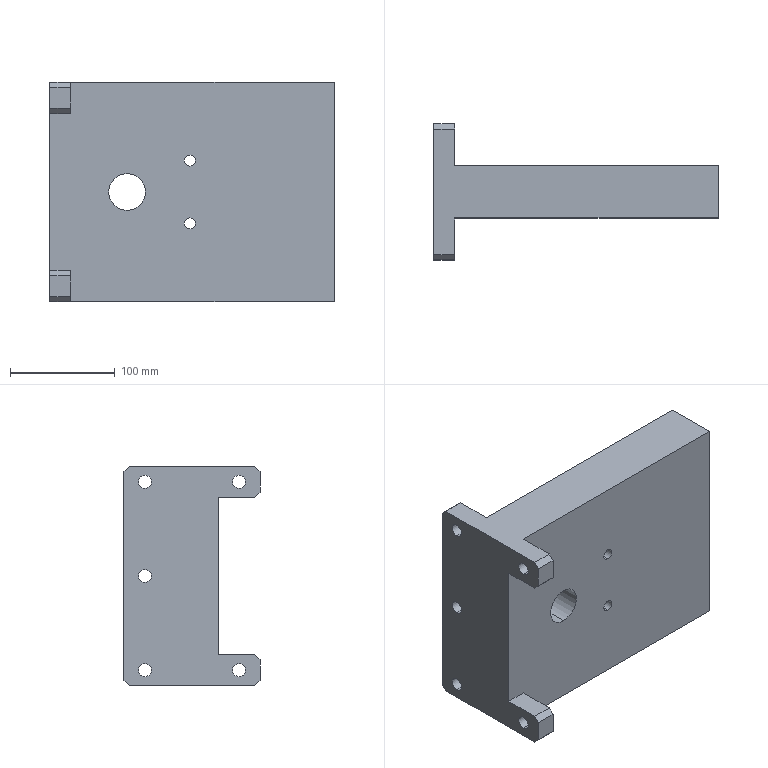Part | SolidWorks | features ICE 5, HoleWzd 3, Chamfer 1, Extrusion 1, Fillet 1 | 1 solid | 53 faces | box 272 x 130 x 210 mm | volume 2006096 mm3 | plane 25 | cylinder 24 | cone 4 | commonest cylinder face diameters 12.5 x10 6.8 x4 10.5 x4 10 x2 35 x2 52 x2